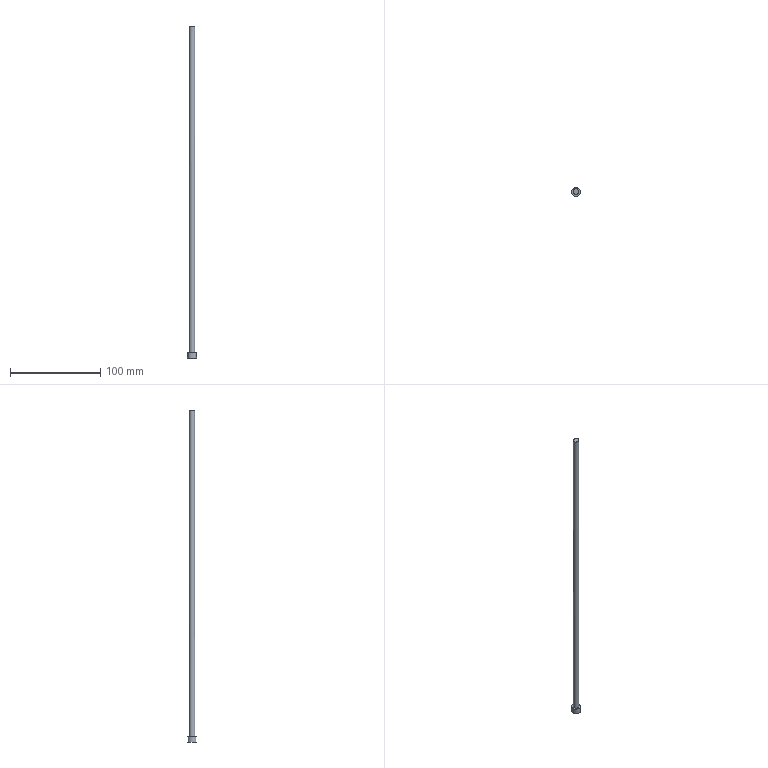Part | NX | features solid 2 | 1 solid | 5 faces | box 10 x 10 x 368.654 mm | volume 10708 mm3 | cylinder 2 | plane 2 | spline 1 | commonest cylinder face diameters 6 x1 10 x1
STEP:
#1=CARTESIAN_POINT('',(26.5,69.,-339.5));
#2=VERTEX_POINT('',#1);
#3=CARTESIAN_POINT('',(29.5,69.,-339.5));
#4=DIRECTION('',(0.,0.,-1.));
#5=DIRECTION('',(-1.,0.,0.));
#6=AXIS2_PLACEMENT_3D('',#3,#4,#5);
#7=CIRCLE('',#6,3.);
#8=EDGE_CURVE('',#2,#2,#7,.T.);
#9=ORIENTED_EDGE('',*,*,#8,.F.);
#10=EDGE_LOOP('',(#9));
#11=FACE_BOUND('',#10,.T.);
#12=CARTESIAN_POINT('',(26.517,68.681,22.127));
#13=VERTEX_POINT('',#12);
#14=CARTESIAN_POINT('',(27.426,66.405,22.322));
#15=CARTESIAN_POINT('',(26.188,68.643,22.067));
#16=CARTESIAN_POINT('',(26.926,71.106,22.171));
#17=CARTESIAN_POINT('',(29.154,72.3,22.552));
#18=CARTESIAN_POINT('',(31.575,71.596,22.969));
#19=CARTESIAN_POINT('',(32.811,69.357,23.199));
#20=CARTESIAN_POINT('',(32.078,66.897,23.111));
#21=CARTESIAN_POINT('',(29.841,65.699,22.754));
#22=CARTESIAN_POINT('',(27.426,66.405,22.322));
#23=CARTESIAN_POINT('',(26.188,68.643,22.067));
#24=CARTESIAN_POINT('',(26.926,71.106,22.171));
#25=B_SPLINE_CURVE_WITH_KNOTS('',3,(#14,#15,#16,#17,#18,#19,#20,#21,#22,#23,#24),.UNSPECIFIED.,.T.,.F.,(1,1,1,1,1,1,1,1,1,1,1,1,1,1,1),(-0.007087,-0.004725,-0.002362,0.,0.002362,0.004725,0.007087,0.009449,0.01181,0.01417,0.01654,0.0189,0.02126,0.02362,0.02599),.UNSPECIFIED.);
#26=EDGE_CURVE('',#13,#13,#25,.T.);
#27=ORIENTED_EDGE('',*,*,#26,.T.);
#28=EDGE_LOOP('',(#27));
#29=FACE_BOUND('',#28,.T.);
#30=CARTESIAN_POINT('',(29.5,69.,-345.5));
#31=DIRECTION('',(0.,0.,1.));
#32=DIRECTION('',(-1.,0.,0.));
#33=AXIS2_PLACEMENT_3D('',#30,#31,#32);
#34=CYLINDRICAL_SURFACE('',#33,3.);
#35=ADVANCED_FACE('',(#11,#29),#34,.T.);
#36=ORIENTED_EDGE('',*,*,#8,.T.);
#37=EDGE_LOOP('',(#36));
#38=FACE_BOUND('',#37,.T.);
#39=CARTESIAN_POINT('',(24.5,69.,-339.5));
#40=VERTEX_POINT('',#39);
#41=CARTESIAN_POINT('',(29.5,69.,-339.5));
#42=DIRECTION('',(0.,0.,1.));
#43=DIRECTION('',(-1.,0.,0.));
#44=AXIS2_PLACEMENT_3D('',#41,#42,#43);
#45=CIRCLE('',#44,5.);
#46=EDGE_CURVE('',#40,#40,#45,.T.);
#47=ORIENTED_EDGE('',*,*,#46,.T.);
#48=EDGE_LOOP('',(#47));
#49=FACE_BOUND('',#48,.T.);
#50=CARTESIAN_POINT('',(29.5,69.,-339.5));
#51=DIRECTION('',(0.,0.,1.));
#52=DIRECTION('',(-1.,0.,0.));
#53=AXIS2_PLACEMENT_3D('',#50,#51,#52);
#54=PLANE('',#53);
#55=ADVANCED_FACE('',(#38,#49),#54,.T.);
#56=CARTESIAN_POINT('',(24.5,69.,-345.5));
#57=VERTEX_POINT('',#56);
#58=CARTESIAN_POINT('',(29.5,69.,-345.5));
#59=DIRECTION('',(0.,0.,-1.));
#60=DIRECTION('',(-1.,0.,0.));
#61=AXIS2_PLACEMENT_3D('',#58,#59,#60);
#62=CIRCLE('',#61,5.);
#63=EDGE_CURVE('',#57,#57,#62,.T.);
#64=ORIENTED_EDGE('',*,*,#63,.T.);
#65=EDGE_LOOP('',(#64));
#66=FACE_BOUND('',#65,.T.);
#67=CARTESIAN_POINT('',(29.5,69.,-345.5));
#68=DIRECTION('',(0.,0.,-1.));
#69=DIRECTION('',(1.,0.,0.));
#70=AXIS2_PLACEMENT_3D('',#67,#68,#69);
#71=PLANE('',#70);
#72=ADVANCED_FACE('',(#66),#71,.T.);
#73=ORIENTED_EDGE('',*,*,#46,.F.);
#74=EDGE_LOOP('',(#73));
#75=FACE_BOUND('',#74,.T.);
#76=ORIENTED_EDGE('',*,*,#63,.F.);
#77=EDGE_LOOP('',(#76));
#78=FACE_BOUND('',#77,.T.);
#79=CARTESIAN_POINT('',(29.5,69.,-345.5));
#80=DIRECTION('',(0.,0.,1.));
#81=DIRECTION('',(-1.,0.,0.));
#82=AXIS2_PLACEMENT_3D('',#79,#80,#81);
#83=CYLINDRICAL_SURFACE('',#82,5.);
#84=ADVANCED_FACE('',(#75,#78),#83,.T.);
#85=ORIENTED_EDGE('',*,*,#26,.F.);
#86=EDGE_LOOP('',(#85));
#87=FACE_BOUND('',#86,.T.);
#88=CARTESIAN_POINT('',(26.437,65.945,22.148));
#89=CARTESIAN_POINT('',(26.443,67.976,22.122));
#90=CARTESIAN_POINT('',(26.449,70.008,22.097));
#91=CARTESIAN_POINT('',(26.455,72.039,22.074));
#92=CARTESIAN_POINT('',(28.469,65.945,22.517));
#93=CARTESIAN_POINT('',(28.475,67.976,22.491));
#94=CARTESIAN_POINT('',(28.48,70.008,22.466));
#95=CARTESIAN_POINT('',(28.486,72.039,22.443));
#96=CARTESIAN_POINT('',(30.506,65.945,22.866));
#97=CARTESIAN_POINT('',(30.511,67.976,22.84));
#98=CARTESIAN_POINT('',(30.517,70.008,22.815));
#99=CARTESIAN_POINT('',(30.523,72.039,22.791));
#100=CARTESIAN_POINT('',(32.547,65.945,23.201));
#101=CARTESIAN_POINT('',(32.552,67.976,23.174));
#102=CARTESIAN_POINT('',(32.557,70.008,23.149));
#103=CARTESIAN_POINT('',(32.563,72.039,23.126));
#104=B_SPLINE_SURFACE_WITH_KNOTS('',3,3,((#88,#89,#90,#91),(#92,#93,#94,#95),(#96,#97,#98,#99),(#100,#101,#102,#103)),.UNSPECIFIED.,.F.,.F.,.F.,(4,4),(4,4),(0.7827,0.8138),(0.8036,0.9193),.PIECEWISE_BEZIER_KNOTS.);
#105=ADVANCED_FACE('',(#87),#104,.T.);
#106=CLOSED_SHELL('',(#35,#55,#72,#84,#105));
#107=MANIFOLD_SOLID_BREP('',#106);
#108=(LENGTH_UNIT()NAMED_UNIT(*)SI_UNIT(.MILLI.,.METRE.));
#109=UNCERTAINTY_MEASURE_WITH_UNIT(LENGTH_MEASURE(0.0508),#108,'','');
#110=(NAMED_UNIT(*)PLANE_ANGLE_UNIT()SI_UNIT($,.RADIAN.));
#111=(NAMED_UNIT(*)SI_UNIT($,.STERADIAN.)SOLID_ANGLE_UNIT());
#112=(GEOMETRIC_REPRESENTATION_CONTEXT(3)GLOBAL_UNCERTAINTY_ASSIGNED_CONTEXT((#109))GLOBAL_UNIT_ASSIGNED_CONTEXT((#108,#110,#111))REPRESENTATION_CONTEXT('',''));
#113=ADVANCED_BREP_SHAPE_REPRESENTATION('',(#107),#112);